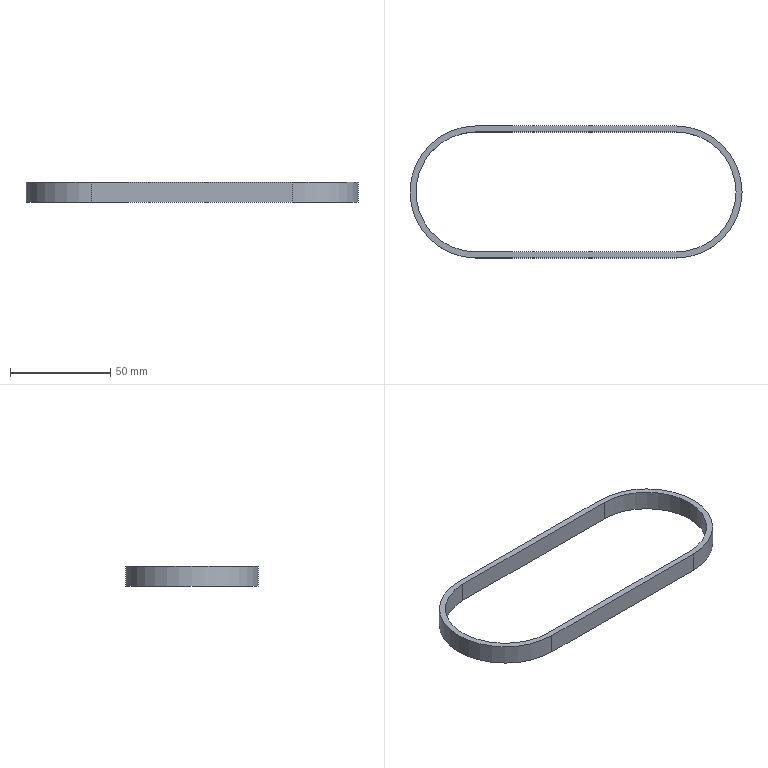Part | SolidWorks | features Extrusion 1 | 1 solid | 12 faces | box 166 x 66 x 10 mm | volume 11938 mm3 | cylinder 6 | plane 6 | commonest cylinder face diameters 60 x3 66 x3
STEP:
#1=CARTESIAN_POINT('',(80.,0.,-5.));
#2=VERTEX_POINT('',#1);
#3=CARTESIAN_POINT('',(50.,30.,-5.));
#4=VERTEX_POINT('',#3);
#5=CARTESIAN_POINT('',(50.,0.,-5.));
#6=DIRECTION('',(0.,0.,1.));
#7=DIRECTION('',(-1.,0.,0.));
#8=AXIS2_PLACEMENT_3D('',#5,#6,#7);
#9=CIRCLE('',#8,30.);
#10=EDGE_CURVE('',#2,#4,#9,.T.);
#11=ORIENTED_EDGE('',*,*,#10,.F.);
#12=CARTESIAN_POINT('',(80.,0.,5.));
#13=VERTEX_POINT('',#12);
#14=CARTESIAN_POINT('',(80.,0.,-5.));
#15=DIRECTION('',(0.,0.,1.));
#16=VECTOR('',#15,1000.);
#17=LINE('',#14,#16);
#18=EDGE_CURVE('',#2,#13,#17,.T.);
#19=ORIENTED_EDGE('',*,*,#18,.T.);
#20=CARTESIAN_POINT('',(50.,30.,5.));
#21=VERTEX_POINT('',#20);
#22=CARTESIAN_POINT('',(50.,0.,5.));
#23=DIRECTION('',(0.,0.,1.));
#24=DIRECTION('',(-1.,0.,0.));
#25=AXIS2_PLACEMENT_3D('',#22,#23,#24);
#26=CIRCLE('',#25,30.);
#27=EDGE_CURVE('',#13,#21,#26,.T.);
#28=ORIENTED_EDGE('',*,*,#27,.T.);
#29=CARTESIAN_POINT('',(50.,30.,-5.));
#30=DIRECTION('',(0.,0.,1.));
#31=VECTOR('',#30,1000.);
#32=LINE('',#29,#31);
#33=EDGE_CURVE('',#4,#21,#32,.T.);
#34=ORIENTED_EDGE('',*,*,#33,.F.);
#35=EDGE_LOOP('',(#11,#19,#28,#34));
#36=FACE_OUTER_BOUND('',#35,.T.);
#37=CARTESIAN_POINT('',(50.,0.,-5.));
#38=DIRECTION('',(0.,0.,1.));
#39=DIRECTION('',(1.,0.,0.));
#40=AXIS2_PLACEMENT_3D('',#37,#38,#39);
#41=CYLINDRICAL_SURFACE('',#40,30.);
#42=ADVANCED_FACE('',(#36),#41,.F.);
#43=CARTESIAN_POINT('',(50.,-33.,-5.));
#44=VERTEX_POINT('',#43);
#45=CARTESIAN_POINT('',(83.,0.,-5.));
#46=VERTEX_POINT('',#45);
#47=CARTESIAN_POINT('',(50.,0.,-5.));
#48=DIRECTION('',(0.,0.,1.));
#49=DIRECTION('',(-1.,0.,0.));
#50=AXIS2_PLACEMENT_3D('',#47,#48,#49);
#51=CIRCLE('',#50,33.);
#52=EDGE_CURVE('',#44,#46,#51,.T.);
#53=ORIENTED_EDGE('',*,*,#52,.T.);
#54=CARTESIAN_POINT('',(83.,0.,5.));
#55=VERTEX_POINT('',#54);
#56=CARTESIAN_POINT('',(83.,0.,-5.));
#57=DIRECTION('',(0.,0.,1.));
#58=VECTOR('',#57,1000.);
#59=LINE('',#56,#58);
#60=EDGE_CURVE('',#46,#55,#59,.T.);
#61=ORIENTED_EDGE('',*,*,#60,.T.);
#62=CARTESIAN_POINT('',(50.,-33.,5.));
#63=VERTEX_POINT('',#62);
#64=CARTESIAN_POINT('',(50.,0.,5.));
#65=DIRECTION('',(0.,0.,1.));
#66=DIRECTION('',(-1.,0.,0.));
#67=AXIS2_PLACEMENT_3D('',#64,#65,#66);
#68=CIRCLE('',#67,33.);
#69=EDGE_CURVE('',#63,#55,#68,.T.);
#70=ORIENTED_EDGE('',*,*,#69,.F.);
#71=CARTESIAN_POINT('',(50.,-33.,-5.));
#72=DIRECTION('',(0.,0.,1.));
#73=VECTOR('',#72,1000.);
#74=LINE('',#71,#73);
#75=EDGE_CURVE('',#44,#63,#74,.T.);
#76=ORIENTED_EDGE('',*,*,#75,.F.);
#77=EDGE_LOOP('',(#53,#61,#70,#76));
#78=FACE_OUTER_BOUND('',#77,.T.);
#79=CARTESIAN_POINT('',(50.,0.,-5.));
#80=DIRECTION('',(0.,0.,1.));
#81=DIRECTION('',(1.,0.,0.));
#82=AXIS2_PLACEMENT_3D('',#79,#80,#81);
#83=CYLINDRICAL_SURFACE('',#82,33.);
#84=ADVANCED_FACE('',(#78),#83,.T.);
#85=CARTESIAN_POINT('',(-50.,33.,5.));
#86=VERTEX_POINT('',#85);
#87=CARTESIAN_POINT('',(-50.,-33.,5.));
#88=VERTEX_POINT('',#87);
#89=CARTESIAN_POINT('',(-50.,0.,5.));
#90=DIRECTION('',(0.,0.,1.));
#91=DIRECTION('',(-1.,0.,0.));
#92=AXIS2_PLACEMENT_3D('',#89,#90,#91);
#93=CIRCLE('',#92,33.);
#94=EDGE_CURVE('',#86,#88,#93,.T.);
#95=ORIENTED_EDGE('',*,*,#94,.F.);
#96=CARTESIAN_POINT('',(-50.,33.,-5.));
#97=VERTEX_POINT('',#96);
#98=CARTESIAN_POINT('',(-50.,33.,-5.));
#99=DIRECTION('',(0.,0.,1.));
#100=VECTOR('',#99,1000.);
#101=LINE('',#98,#100);
#102=EDGE_CURVE('',#97,#86,#101,.T.);
#103=ORIENTED_EDGE('',*,*,#102,.F.);
#104=CARTESIAN_POINT('',(-50.,-33.,-5.));
#105=VERTEX_POINT('',#104);
#106=CARTESIAN_POINT('',(-50.,0.,-5.));
#107=DIRECTION('',(0.,0.,1.));
#108=DIRECTION('',(-1.,0.,0.));
#109=AXIS2_PLACEMENT_3D('',#106,#107,#108);
#110=CIRCLE('',#109,33.);
#111=EDGE_CURVE('',#97,#105,#110,.T.);
#112=ORIENTED_EDGE('',*,*,#111,.T.);
#113=CARTESIAN_POINT('',(-50.,-33.,-5.));
#114=DIRECTION('',(0.,0.,1.));
#115=VECTOR('',#114,1000.);
#116=LINE('',#113,#115);
#117=EDGE_CURVE('',#105,#88,#116,.T.);
#118=ORIENTED_EDGE('',*,*,#117,.T.);
#119=EDGE_LOOP('',(#95,#103,#112,#118));
#120=FACE_OUTER_BOUND('',#119,.T.);
#121=CARTESIAN_POINT('',(-50.,0.,-5.));
#122=DIRECTION('',(0.,0.,1.));
#123=DIRECTION('',(1.,0.,0.));
#124=AXIS2_PLACEMENT_3D('',#121,#122,#123);
#125=CYLINDRICAL_SURFACE('',#124,33.);
#126=ADVANCED_FACE('',(#120),#125,.T.);
#127=CARTESIAN_POINT('',(50.,33.,5.));
#128=VERTEX_POINT('',#127);
#129=CARTESIAN_POINT('',(-50.,33.,5.));
#130=DIRECTION('',(-1.,0.,0.));
#131=VECTOR('',#130,1000.);
#132=LINE('',#129,#131);
#133=EDGE_CURVE('',#128,#86,#132,.T.);
#134=ORIENTED_EDGE('',*,*,#133,.F.);
#135=CARTESIAN_POINT('',(50.,33.,-5.));
#136=VERTEX_POINT('',#135);
#137=CARTESIAN_POINT('',(50.,33.,-5.));
#138=DIRECTION('',(0.,0.,1.));
#139=VECTOR('',#138,1000.);
#140=LINE('',#137,#139);
#141=EDGE_CURVE('',#136,#128,#140,.T.);
#142=ORIENTED_EDGE('',*,*,#141,.F.);
#143=CARTESIAN_POINT('',(-50.,33.,-5.));
#144=DIRECTION('',(-1.,0.,0.));
#145=VECTOR('',#144,1000.);
#146=LINE('',#143,#145);
#147=EDGE_CURVE('',#136,#97,#146,.T.);
#148=ORIENTED_EDGE('',*,*,#147,.T.);
#149=ORIENTED_EDGE('',*,*,#102,.T.);
#150=EDGE_LOOP('',(#134,#142,#148,#149));
#151=FACE_OUTER_BOUND('',#150,.T.);
#152=CARTESIAN_POINT('',(-50.,33.,-5.));
#153=DIRECTION('',(0.,1.,0.));
#154=DIRECTION('',(0.,0.,1.));
#155=AXIS2_PLACEMENT_3D('',#152,#153,#154);
#156=PLANE('',#155);
#157=ADVANCED_FACE('',(#151),#156,.T.);
#158=ORIENTED_EDGE('',*,*,#60,.F.);
#159=CARTESIAN_POINT('',(50.,0.,-5.));
#160=DIRECTION('',(0.,0.,1.));
#161=DIRECTION('',(-1.,0.,0.));
#162=AXIS2_PLACEMENT_3D('',#159,#160,#161);
#163=CIRCLE('',#162,33.);
#164=EDGE_CURVE('',#46,#136,#163,.T.);
#165=ORIENTED_EDGE('',*,*,#164,.T.);
#166=ORIENTED_EDGE('',*,*,#141,.T.);
#167=CARTESIAN_POINT('',(50.,0.,5.));
#168=DIRECTION('',(0.,0.,1.));
#169=DIRECTION('',(-1.,0.,0.));
#170=AXIS2_PLACEMENT_3D('',#167,#168,#169);
#171=CIRCLE('',#170,33.);
#172=EDGE_CURVE('',#55,#128,#171,.T.);
#173=ORIENTED_EDGE('',*,*,#172,.F.);
#174=EDGE_LOOP('',(#158,#165,#166,#173));
#175=FACE_OUTER_BOUND('',#174,.T.);
#176=CARTESIAN_POINT('',(50.,0.,-5.));
#177=DIRECTION('',(0.,0.,1.));
#178=DIRECTION('',(1.,0.,0.));
#179=AXIS2_PLACEMENT_3D('',#176,#177,#178);
#180=CYLINDRICAL_SURFACE('',#179,33.);
#181=ADVANCED_FACE('',(#175),#180,.T.);
#182=CARTESIAN_POINT('',(50.,-33.,5.));
#183=DIRECTION('',(1.,0.,0.));
#184=VECTOR('',#183,1000.);
#185=LINE('',#182,#184);
#186=EDGE_CURVE('',#88,#63,#185,.T.);
#187=ORIENTED_EDGE('',*,*,#186,.F.);
#188=ORIENTED_EDGE('',*,*,#117,.F.);
#189=CARTESIAN_POINT('',(50.,-33.,-5.));
#190=DIRECTION('',(1.,0.,0.));
#191=VECTOR('',#190,1000.);
#192=LINE('',#189,#191);
#193=EDGE_CURVE('',#105,#44,#192,.T.);
#194=ORIENTED_EDGE('',*,*,#193,.T.);
#195=ORIENTED_EDGE('',*,*,#75,.T.);
#196=EDGE_LOOP('',(#187,#188,#194,#195));
#197=FACE_OUTER_BOUND('',#196,.T.);
#198=CARTESIAN_POINT('',(50.,-33.,-5.));
#199=DIRECTION('',(0.,-1.,0.));
#200=DIRECTION('',(0.,0.,-1.));
#201=AXIS2_PLACEMENT_3D('',#198,#199,#200);
#202=PLANE('',#201);
#203=ADVANCED_FACE('',(#197),#202,.T.);
#204=CARTESIAN_POINT('',(-50.,30.,-5.));
#205=VERTEX_POINT('',#204);
#206=CARTESIAN_POINT('',(-50.,-30.,-5.));
#207=VERTEX_POINT('',#206);
#208=CARTESIAN_POINT('',(-50.,0.,-5.));
#209=DIRECTION('',(0.,0.,1.));
#210=DIRECTION('',(-1.,0.,0.));
#211=AXIS2_PLACEMENT_3D('',#208,#209,#210);
#212=CIRCLE('',#211,30.);
#213=EDGE_CURVE('',#205,#207,#212,.T.);
#214=ORIENTED_EDGE('',*,*,#213,.T.);
#215=CARTESIAN_POINT('',(50.,-30.,-5.));
#216=VERTEX_POINT('',#215);
#217=CARTESIAN_POINT('',(50.,-30.,-5.));
#218=DIRECTION('',(1.,0.,0.));
#219=VECTOR('',#218,1000.);
#220=LINE('',#217,#219);
#221=EDGE_CURVE('',#207,#216,#220,.T.);
#222=ORIENTED_EDGE('',*,*,#221,.T.);
#223=CARTESIAN_POINT('',(50.,0.,-5.));
#224=DIRECTION('',(0.,0.,1.));
#225=DIRECTION('',(-1.,0.,0.));
#226=AXIS2_PLACEMENT_3D('',#223,#224,#225);
#227=CIRCLE('',#226,30.);
#228=EDGE_CURVE('',#216,#2,#227,.T.);
#229=ORIENTED_EDGE('',*,*,#228,.T.);
#230=ORIENTED_EDGE('',*,*,#10,.T.);
#231=CARTESIAN_POINT('',(-50.,30.,-5.));
#232=DIRECTION('',(-1.,0.,0.));
#233=VECTOR('',#232,1000.);
#234=LINE('',#231,#233);
#235=EDGE_CURVE('',#4,#205,#234,.T.);
#236=ORIENTED_EDGE('',*,*,#235,.T.);
#237=EDGE_LOOP('',(#214,#222,#229,#230,#236));
#238=FACE_BOUND('',#237,.T.);
#239=ORIENTED_EDGE('',*,*,#111,.F.);
#240=ORIENTED_EDGE('',*,*,#147,.F.);
#241=ORIENTED_EDGE('',*,*,#164,.F.);
#242=ORIENTED_EDGE('',*,*,#52,.F.);
#243=ORIENTED_EDGE('',*,*,#193,.F.);
#244=EDGE_LOOP('',(#239,#240,#241,#242,#243));
#245=FACE_OUTER_BOUND('',#244,.T.);
#246=CARTESIAN_POINT('',(-50.,0.,-5.));
#247=DIRECTION('',(0.,0.,-1.));
#248=DIRECTION('',(-1.,0.,0.));
#249=AXIS2_PLACEMENT_3D('',#246,#247,#248);
#250=PLANE('',#249);
#251=ADVANCED_FACE('',(#238,#245),#250,.T.);
#252=CARTESIAN_POINT('',(-50.,-30.,5.));
#253=VERTEX_POINT('',#252);
#254=CARTESIAN_POINT('',(50.,-30.,5.));
#255=VERTEX_POINT('',#254);
#256=CARTESIAN_POINT('',(50.,-30.,5.));
#257=DIRECTION('',(1.,0.,0.));
#258=VECTOR('',#257,1000.);
#259=LINE('',#256,#258);
#260=EDGE_CURVE('',#253,#255,#259,.T.);
#261=ORIENTED_EDGE('',*,*,#260,.F.);
#262=CARTESIAN_POINT('',(-50.,30.,5.));
#263=VERTEX_POINT('',#262);
#264=CARTESIAN_POINT('',(-50.,0.,5.));
#265=DIRECTION('',(0.,0.,1.));
#266=DIRECTION('',(-1.,0.,0.));
#267=AXIS2_PLACEMENT_3D('',#264,#265,#266);
#268=CIRCLE('',#267,30.);
#269=EDGE_CURVE('',#263,#253,#268,.T.);
#270=ORIENTED_EDGE('',*,*,#269,.F.);
#271=CARTESIAN_POINT('',(-50.,30.,5.));
#272=DIRECTION('',(-1.,0.,0.));
#273=VECTOR('',#272,1000.);
#274=LINE('',#271,#273);
#275=EDGE_CURVE('',#21,#263,#274,.T.);
#276=ORIENTED_EDGE('',*,*,#275,.F.);
#277=ORIENTED_EDGE('',*,*,#27,.F.);
#278=CARTESIAN_POINT('',(50.,0.,5.));
#279=DIRECTION('',(0.,0.,1.));
#280=DIRECTION('',(-1.,0.,0.));
#281=AXIS2_PLACEMENT_3D('',#278,#279,#280);
#282=CIRCLE('',#281,30.);
#283=EDGE_CURVE('',#255,#13,#282,.T.);
#284=ORIENTED_EDGE('',*,*,#283,.F.);
#285=EDGE_LOOP('',(#261,#270,#276,#277,#284));
#286=FACE_BOUND('',#285,.T.);
#287=ORIENTED_EDGE('',*,*,#94,.T.);
#288=ORIENTED_EDGE('',*,*,#186,.T.);
#289=ORIENTED_EDGE('',*,*,#69,.T.);
#290=ORIENTED_EDGE('',*,*,#172,.T.);
#291=ORIENTED_EDGE('',*,*,#133,.T.);
#292=EDGE_LOOP('',(#287,#288,#289,#290,#291));
#293=FACE_OUTER_BOUND('',#292,.T.);
#294=CARTESIAN_POINT('',(-50.,0.,5.));
#295=DIRECTION('',(0.,0.,-1.));
#296=DIRECTION('',(-1.,0.,0.));
#297=AXIS2_PLACEMENT_3D('',#294,#295,#296);
#298=PLANE('',#297);
#299=ADVANCED_FACE('',(#286,#293),#298,.F.);
#300=ORIENTED_EDGE('',*,*,#269,.T.);
#301=CARTESIAN_POINT('',(-50.,-30.,-5.));
#302=DIRECTION('',(0.,0.,1.));
#303=VECTOR('',#302,1000.);
#304=LINE('',#301,#303);
#305=EDGE_CURVE('',#207,#253,#304,.T.);
#306=ORIENTED_EDGE('',*,*,#305,.F.);
#307=ORIENTED_EDGE('',*,*,#213,.F.);
#308=CARTESIAN_POINT('',(-50.,30.,-5.));
#309=DIRECTION('',(0.,0.,1.));
#310=VECTOR('',#309,1000.);
#311=LINE('',#308,#310);
#312=EDGE_CURVE('',#205,#263,#311,.T.);
#313=ORIENTED_EDGE('',*,*,#312,.T.);
#314=EDGE_LOOP('',(#300,#306,#307,#313));
#315=FACE_OUTER_BOUND('',#314,.T.);
#316=CARTESIAN_POINT('',(-50.,0.,-5.));
#317=DIRECTION('',(0.,0.,1.));
#318=DIRECTION('',(1.,0.,0.));
#319=AXIS2_PLACEMENT_3D('',#316,#317,#318);
#320=CYLINDRICAL_SURFACE('',#319,30.);
#321=ADVANCED_FACE('',(#315),#320,.F.);
#322=ORIENTED_EDGE('',*,*,#275,.T.);
#323=ORIENTED_EDGE('',*,*,#312,.F.);
#324=ORIENTED_EDGE('',*,*,#235,.F.);
#325=ORIENTED_EDGE('',*,*,#33,.T.);
#326=EDGE_LOOP('',(#322,#323,#324,#325));
#327=FACE_OUTER_BOUND('',#326,.T.);
#328=CARTESIAN_POINT('',(-50.,30.,-5.));
#329=DIRECTION('',(0.,1.,0.));
#330=DIRECTION('',(0.,0.,1.));
#331=AXIS2_PLACEMENT_3D('',#328,#329,#330);
#332=PLANE('',#331);
#333=ADVANCED_FACE('',(#327),#332,.F.);
#334=ORIENTED_EDGE('',*,*,#18,.F.);
#335=ORIENTED_EDGE('',*,*,#228,.F.);
#336=CARTESIAN_POINT('',(50.,-30.,-5.));
#337=DIRECTION('',(0.,0.,1.));
#338=VECTOR('',#337,1000.);
#339=LINE('',#336,#338);
#340=EDGE_CURVE('',#216,#255,#339,.T.);
#341=ORIENTED_EDGE('',*,*,#340,.T.);
#342=ORIENTED_EDGE('',*,*,#283,.T.);
#343=EDGE_LOOP('',(#334,#335,#341,#342));
#344=FACE_OUTER_BOUND('',#343,.T.);
#345=CARTESIAN_POINT('',(50.,0.,-5.));
#346=DIRECTION('',(0.,0.,1.));
#347=DIRECTION('',(1.,0.,0.));
#348=AXIS2_PLACEMENT_3D('',#345,#346,#347);
#349=CYLINDRICAL_SURFACE('',#348,30.);
#350=ADVANCED_FACE('',(#344),#349,.F.);
#351=ORIENTED_EDGE('',*,*,#260,.T.);
#352=ORIENTED_EDGE('',*,*,#340,.F.);
#353=ORIENTED_EDGE('',*,*,#221,.F.);
#354=ORIENTED_EDGE('',*,*,#305,.T.);
#355=EDGE_LOOP('',(#351,#352,#353,#354));
#356=FACE_OUTER_BOUND('',#355,.T.);
#357=CARTESIAN_POINT('',(50.,-30.,-5.));
#358=DIRECTION('',(0.,-1.,0.));
#359=DIRECTION('',(0.,0.,-1.));
#360=AXIS2_PLACEMENT_3D('',#357,#358,#359);
#361=PLANE('',#360);
#362=ADVANCED_FACE('',(#356),#361,.F.);
#363=CLOSED_SHELL('',(#42,#84,#126,#157,#181,#203,#251,#299,#321,#333,#350,#362));
#364=MANIFOLD_SOLID_BREP('',#363);
#365=CARTESIAN_POINT('',(0.,0.,0.));
#366=DIRECTION('',(0.,0.,1.));
#367=DIRECTION('',(1.,0.,0.));
#368=AXIS2_PLACEMENT_3D('',#365,#366,#367);
#369=(LENGTH_UNIT()NAMED_UNIT(*)SI_UNIT(.MILLI.,.METRE.));
#370=UNCERTAINTY_MEASURE_WITH_UNIT(LENGTH_MEASURE(0.00001),#369,'','');
#371=(NAMED_UNIT(*)PLANE_ANGLE_UNIT()SI_UNIT($,.RADIAN.));
#372=(NAMED_UNIT(*)SI_UNIT($,.STERADIAN.)SOLID_ANGLE_UNIT());
#373=(GEOMETRIC_REPRESENTATION_CONTEXT(3)GLOBAL_UNCERTAINTY_ASSIGNED_CONTEXT((#370))GLOBAL_UNIT_ASSIGNED_CONTEXT((#369,#371,#372))REPRESENTATION_CONTEXT('',''));
#374=ADVANCED_BREP_SHAPE_REPRESENTATION('',(#364,#368),#373);